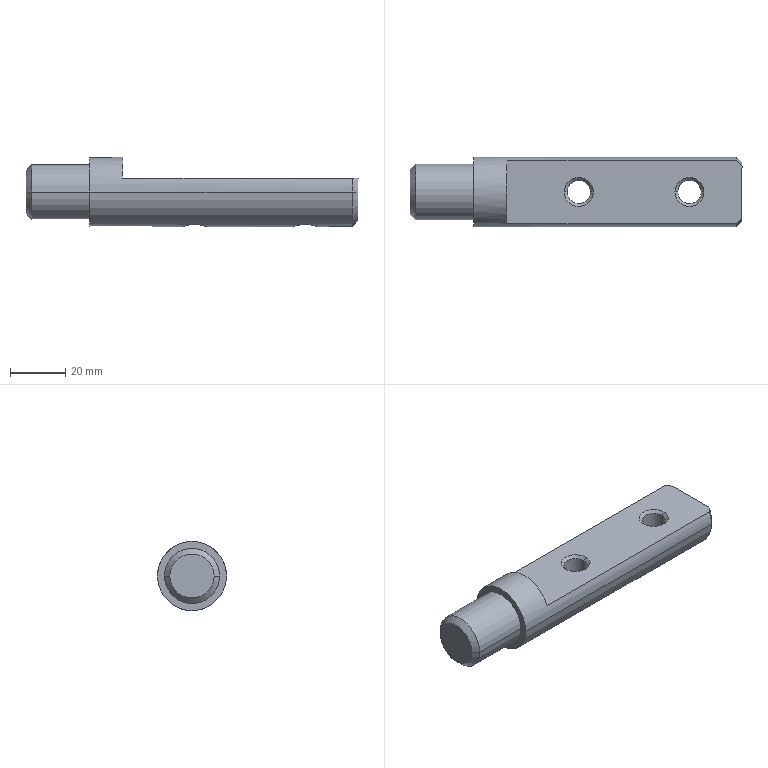Part | SolidWorks | features Chamfer 2, HoleWzd 1, ICE 1, Revolution 1 | 1 solid | 22 faces | box 120 x 25 x 25 mm | volume 42106 mm3 | cone 9 | cylinder 8 | plane 5 | commonest cylinder face diameters 8.5 x4 20 x2 25 x2
STEP:
#1=CARTESIAN_POINT('',(56.75,0.,4.));
#2=VERTEX_POINT('',#1);
#3=CARTESIAN_POINT('',(65.25,0.,4.));
#4=VERTEX_POINT('',#3);
#5=CARTESIAN_POINT('',(61.,0.,4.));
#6=DIRECTION('',(0.,0.,1.));
#7=DIRECTION('',(1.,0.,0.));
#8=AXIS2_PLACEMENT_3D('',#5,#6,#7);
#9=CIRCLE('',#8,4.25);
#10=EDGE_CURVE('',#2,#4,#9,.T.);
#11=ORIENTED_EDGE('',*,*,#10,.F.);
#12=CARTESIAN_POINT('',(55.75,0.,5.));
#13=VERTEX_POINT('',#12);
#14=CARTESIAN_POINT('',(56.75,0.,4.));
#15=DIRECTION('',(-0.7071,0.,0.7071));
#16=VECTOR('',#15,1000.);
#17=LINE('',#14,#16);
#18=EDGE_CURVE('',#2,#13,#17,.T.);
#19=ORIENTED_EDGE('',*,*,#18,.T.);
#20=CARTESIAN_POINT('',(66.25,0.,5.));
#21=VERTEX_POINT('',#20);
#22=CARTESIAN_POINT('',(61.,0.,5.));
#23=DIRECTION('',(0.,0.,-1.));
#24=DIRECTION('',(1.,0.,0.));
#25=AXIS2_PLACEMENT_3D('',#22,#23,#24);
#26=CIRCLE('',#25,5.25);
#27=EDGE_CURVE('',#21,#13,#26,.T.);
#28=ORIENTED_EDGE('',*,*,#27,.F.);
#29=CARTESIAN_POINT('',(65.25,0.,4.));
#30=DIRECTION('',(0.7071,0.,0.7071));
#31=VECTOR('',#30,1000.);
#32=LINE('',#29,#31);
#33=EDGE_CURVE('',#4,#21,#32,.T.);
#34=ORIENTED_EDGE('',*,*,#33,.F.);
#35=EDGE_LOOP('',(#11,#19,#28,#34));
#36=FACE_OUTER_BOUND('',#35,.T.);
#37=CARTESIAN_POINT('',(61.,0.,4.));
#38=DIRECTION('',(0.,0.,1.));
#39=DIRECTION('',(1.,0.,0.));
#40=AXIS2_PLACEMENT_3D('',#37,#38,#39);
#41=CONICAL_SURFACE('',#40,4.25,0.7854);
#42=ADVANCED_FACE('',(#36),#41,.F.);
#43=CARTESIAN_POINT('',(96.75,0.,4.));
#44=VERTEX_POINT('',#43);
#45=CARTESIAN_POINT('',(105.25,0.,4.));
#46=VERTEX_POINT('',#45);
#47=CARTESIAN_POINT('',(101.,0.,4.));
#48=DIRECTION('',(0.,0.,1.));
#49=DIRECTION('',(1.,0.,0.));
#50=AXIS2_PLACEMENT_3D('',#47,#48,#49);
#51=CIRCLE('',#50,4.25);
#52=EDGE_CURVE('',#44,#46,#51,.T.);
#53=ORIENTED_EDGE('',*,*,#52,.F.);
#54=CARTESIAN_POINT('',(95.75,0.,5.));
#55=VERTEX_POINT('',#54);
#56=CARTESIAN_POINT('',(96.75,0.,4.));
#57=DIRECTION('',(-0.7071,0.,0.7071));
#58=VECTOR('',#57,1000.);
#59=LINE('',#56,#58);
#60=EDGE_CURVE('',#44,#55,#59,.T.);
#61=ORIENTED_EDGE('',*,*,#60,.T.);
#62=CARTESIAN_POINT('',(106.25,0.,5.));
#63=VERTEX_POINT('',#62);
#64=CARTESIAN_POINT('',(101.,0.,5.));
#65=DIRECTION('',(0.,0.,-1.));
#66=DIRECTION('',(1.,0.,0.));
#67=AXIS2_PLACEMENT_3D('',#64,#65,#66);
#68=CIRCLE('',#67,5.25);
#69=EDGE_CURVE('',#63,#55,#68,.T.);
#70=ORIENTED_EDGE('',*,*,#69,.F.);
#71=CARTESIAN_POINT('',(105.25,0.,4.));
#72=DIRECTION('',(0.7071,0.,0.7071));
#73=VECTOR('',#72,1000.);
#74=LINE('',#71,#73);
#75=EDGE_CURVE('',#46,#63,#74,.T.);
#76=ORIENTED_EDGE('',*,*,#75,.F.);
#77=EDGE_LOOP('',(#53,#61,#70,#76));
#78=FACE_OUTER_BOUND('',#77,.T.);
#79=CARTESIAN_POINT('',(101.,0.,4.));
#80=DIRECTION('',(0.,0.,1.));
#81=DIRECTION('',(1.,0.,0.));
#82=AXIS2_PLACEMENT_3D('',#79,#80,#81);
#83=CONICAL_SURFACE('',#82,4.25,0.7854);
#84=ADVANCED_FACE('',(#78),#83,.F.);
#85=CARTESIAN_POINT('',(65.25,0.,-12.5));
#86=VERTEX_POINT('',#85);
#87=CARTESIAN_POINT('',(56.75,0.,-12.5));
#88=VERTEX_POINT('',#87);
#89=CARTESIAN_POINT('',(65.25,0.,-12.5));
#90=CARTESIAN_POINT('',(65.25,-0.2831,-12.5));
#91=CARTESIAN_POINT('',(65.222,-0.561,-12.49));
#92=CARTESIAN_POINT('',(65.113,-1.107,-12.454));
#93=CARTESIAN_POINT('',(65.03,-1.378,-12.426));
#94=CARTESIAN_POINT('',(64.816,-1.892,-12.359));
#95=CARTESIAN_POINT('',(64.685,-2.136,-12.318));
#96=CARTESIAN_POINT('',(64.376,-2.596,-12.23));
#97=CARTESIAN_POINT('',(64.198,-2.812,-12.181));
#98=CARTESIAN_POINT('',(63.809,-3.201,-12.085));
#99=CARTESIAN_POINT('',(63.597,-3.376,-12.037));
#100=CARTESIAN_POINT('',(63.133,-3.687,-11.945));
#101=CARTESIAN_POINT('',(62.889,-3.817,-11.903));
#102=CARTESIAN_POINT('',(62.379,-4.03,-11.833));
#103=CARTESIAN_POINT('',(62.109,-4.112,-11.804));
#104=CARTESIAN_POINT('',(61.559,-4.222,-11.765));
#105=CARTESIAN_POINT('',(61.282,-4.25,-11.755));
#106=CARTESIAN_POINT('',(60.723,-4.25,-11.755));
#107=CARTESIAN_POINT('',(60.439,-4.222,-11.766));
#108=CARTESIAN_POINT('',(59.892,-4.112,-11.804));
#109=CARTESIAN_POINT('',(59.626,-4.031,-11.833));
#110=CARTESIAN_POINT('',(59.108,-3.816,-11.904));
#111=CARTESIAN_POINT('',(58.864,-3.684,-11.946));
#112=CARTESIAN_POINT('',(58.405,-3.377,-12.036));
#113=CARTESIAN_POINT('',(58.189,-3.2,-12.085));
#114=CARTESIAN_POINT('',(57.798,-2.808,-12.182));
#115=CARTESIAN_POINT('',(57.624,-2.596,-12.23));
#116=CARTESIAN_POINT('',(57.316,-2.137,-12.318));
#117=CARTESIAN_POINT('',(57.182,-1.888,-12.359));
#118=CARTESIAN_POINT('',(56.97,-1.376,-12.427));
#119=CARTESIAN_POINT('',(56.888,-1.111,-12.454));
#120=CARTESIAN_POINT('',(56.778,-0.5605,-12.49));
#121=CARTESIAN_POINT('',(56.75,-0.2789,-12.5));
#122=CARTESIAN_POINT('',(56.75,0.,-12.5));
#123=B_SPLINE_CURVE_WITH_KNOTS('',3,(#89,#90,#91,#92,#93,#94,#95,#96,#97,#98,#99,#100,#101,#102,#103,#104,#105,#106,#107,#108,#109,#110,#111,#112,#113,#114,#115,#116,#117,#118,#119,#120,#121,#122),.UNSPECIFIED.,.F.,.F.,(4,2,2,2,2,2,2,2,2,2,2,2,2,2,2,2,4),(0.,0.0008368,0.001674,0.00251,0.003347,0.004184,0.005021,0.005857,0.006694,0.007531,0.008368,0.009204,0.01004,0.01088,0.01171,0.01255,0.01339),.UNSPECIFIED.);
#124=EDGE_CURVE('',#86,#88,#123,.T.);
#125=ORIENTED_EDGE('',*,*,#124,.T.);
#126=CARTESIAN_POINT('',(56.75,0.,5.));
#127=DIRECTION('',(0.,0.,1.));
#128=VECTOR('',#127,1000.);
#129=LINE('',#126,#128);
#130=EDGE_CURVE('',#88,#2,#129,.T.);
#131=ORIENTED_EDGE('',*,*,#130,.T.);
#132=ORIENTED_EDGE('',*,*,#10,.T.);
#133=CARTESIAN_POINT('',(65.25,0.,5.));
#134=DIRECTION('',(0.,0.,1.));
#135=VECTOR('',#134,1000.);
#136=LINE('',#133,#135);
#137=EDGE_CURVE('',#86,#4,#136,.T.);
#138=ORIENTED_EDGE('',*,*,#137,.F.);
#139=EDGE_LOOP('',(#125,#131,#132,#138));
#140=FACE_OUTER_BOUND('',#139,.T.);
#141=CARTESIAN_POINT('',(61.,0.,5.));
#142=DIRECTION('',(0.,0.,1.));
#143=DIRECTION('',(1.,0.,0.));
#144=AXIS2_PLACEMENT_3D('',#141,#142,#143);
#145=CYLINDRICAL_SURFACE('',#144,4.25);
#146=ADVANCED_FACE('',(#140),#145,.F.);
#147=CARTESIAN_POINT('',(105.25,0.,-12.5));
#148=VERTEX_POINT('',#147);
#149=CARTESIAN_POINT('',(96.75,0.,-12.5));
#150=VERTEX_POINT('',#149);
#151=CARTESIAN_POINT('',(105.25,0.,-12.5));
#152=CARTESIAN_POINT('',(105.25,-0.2831,-12.5));
#153=CARTESIAN_POINT('',(105.222,-0.561,-12.49));
#154=CARTESIAN_POINT('',(105.113,-1.107,-12.454));
#155=CARTESIAN_POINT('',(105.03,-1.378,-12.426));
#156=CARTESIAN_POINT('',(104.816,-1.892,-12.359));
#157=CARTESIAN_POINT('',(104.685,-2.136,-12.318));
#158=CARTESIAN_POINT('',(104.376,-2.596,-12.23));
#159=CARTESIAN_POINT('',(104.198,-2.812,-12.181));
#160=CARTESIAN_POINT('',(103.809,-3.201,-12.085));
#161=CARTESIAN_POINT('',(103.597,-3.376,-12.037));
#162=CARTESIAN_POINT('',(103.133,-3.687,-11.945));
#163=CARTESIAN_POINT('',(102.889,-3.817,-11.903));
#164=CARTESIAN_POINT('',(102.379,-4.03,-11.833));
#165=CARTESIAN_POINT('',(102.109,-4.112,-11.804));
#166=CARTESIAN_POINT('',(101.559,-4.222,-11.765));
#167=CARTESIAN_POINT('',(101.282,-4.25,-11.755));
#168=CARTESIAN_POINT('',(100.723,-4.25,-11.755));
#169=CARTESIAN_POINT('',(100.439,-4.222,-11.766));
#170=CARTESIAN_POINT('',(99.892,-4.112,-11.804));
#171=CARTESIAN_POINT('',(99.626,-4.031,-11.833));
#172=CARTESIAN_POINT('',(99.108,-3.816,-11.904));
#173=CARTESIAN_POINT('',(98.864,-3.684,-11.946));
#174=CARTESIAN_POINT('',(98.405,-3.377,-12.036));
#175=CARTESIAN_POINT('',(98.189,-3.2,-12.085));
#176=CARTESIAN_POINT('',(97.798,-2.808,-12.182));
#177=CARTESIAN_POINT('',(97.624,-2.596,-12.23));
#178=CARTESIAN_POINT('',(97.316,-2.137,-12.318));
#179=CARTESIAN_POINT('',(97.182,-1.888,-12.359));
#180=CARTESIAN_POINT('',(96.97,-1.376,-12.427));
#181=CARTESIAN_POINT('',(96.888,-1.111,-12.454));
#182=CARTESIAN_POINT('',(96.778,-0.5605,-12.49));
#183=CARTESIAN_POINT('',(96.75,-0.2789,-12.5));
#184=CARTESIAN_POINT('',(96.75,0.,-12.5));
#185=B_SPLINE_CURVE_WITH_KNOTS('',3,(#151,#152,#153,#154,#155,#156,#157,#158,#159,#160,#161,#162,#163,#164,#165,#166,#167,#168,#169,#170,#171,#172,#173,#174,#175,#176,#177,#178,#179,#180,#181,#182,#183,#184),.UNSPECIFIED.,.F.,.F.,(4,2,2,2,2,2,2,2,2,2,2,2,2,2,2,2,4),(0.,0.0008368,0.001674,0.00251,0.003347,0.004184,0.005021,0.005857,0.006694,0.007531,0.008368,0.009204,0.01004,0.01088,0.01171,0.01255,0.01339),.UNSPECIFIED.);
#186=EDGE_CURVE('',#148,#150,#185,.T.);
#187=ORIENTED_EDGE('',*,*,#186,.T.);
#188=CARTESIAN_POINT('',(96.75,0.,5.));
#189=DIRECTION('',(0.,0.,1.));
#190=VECTOR('',#189,1000.);
#191=LINE('',#188,#190);
#192=EDGE_CURVE('',#150,#44,#191,.T.);
#193=ORIENTED_EDGE('',*,*,#192,.T.);
#194=ORIENTED_EDGE('',*,*,#52,.T.);
#195=CARTESIAN_POINT('',(105.25,0.,5.));
#196=DIRECTION('',(0.,0.,1.));
#197=VECTOR('',#196,1000.);
#198=LINE('',#195,#197);
#199=EDGE_CURVE('',#148,#46,#198,.T.);
#200=ORIENTED_EDGE('',*,*,#199,.F.);
#201=EDGE_LOOP('',(#187,#193,#194,#200));
#202=FACE_OUTER_BOUND('',#201,.T.);
#203=CARTESIAN_POINT('',(101.,0.,5.));
#204=DIRECTION('',(0.,0.,1.));
#205=DIRECTION('',(1.,0.,0.));
#206=AXIS2_PLACEMENT_3D('',#203,#204,#205);
#207=CYLINDRICAL_SURFACE('',#206,4.25);
#208=ADVANCED_FACE('',(#202),#207,.F.);
#209=CARTESIAN_POINT('',(0.,-8.,0.));
#210=VERTEX_POINT('',#209);
#211=CARTESIAN_POINT('',(0.,8.,0.));
#212=VERTEX_POINT('',#211);
#213=CARTESIAN_POINT('',(0.,0.,0.));
#214=DIRECTION('',(-1.,0.,0.));
#215=DIRECTION('',(0.,-1.,0.));
#216=AXIS2_PLACEMENT_3D('',#213,#214,#215);
#217=CIRCLE('',#216,8.);
#218=EDGE_CURVE('',#210,#212,#217,.T.);
#219=ORIENTED_EDGE('',*,*,#218,.F.);
#220=CARTESIAN_POINT('',(2.,-10.,0.));
#221=VERTEX_POINT('',#220);
#222=CARTESIAN_POINT('',(2.,-10.,0.));
#223=DIRECTION('',(0.7071,-0.7071,0.));
#224=VECTOR('',#223,1000.);
#225=LINE('',#222,#224);
#226=EDGE_CURVE('',#210,#221,#225,.T.);
#227=ORIENTED_EDGE('',*,*,#226,.T.);
#228=CARTESIAN_POINT('',(2.,10.,0.));
#229=VERTEX_POINT('',#228);
#230=CARTESIAN_POINT('',(2.,0.,0.));
#231=DIRECTION('',(1.,0.,0.));
#232=DIRECTION('',(0.,-1.,0.));
#233=AXIS2_PLACEMENT_3D('',#230,#231,#232);
#234=CIRCLE('',#233,10.);
#235=EDGE_CURVE('',#229,#221,#234,.T.);
#236=ORIENTED_EDGE('',*,*,#235,.F.);
#237=CARTESIAN_POINT('',(2.,10.,0.));
#238=DIRECTION('',(0.7071,0.7071,0.));
#239=VECTOR('',#238,1000.);
#240=LINE('',#237,#239);
#241=EDGE_CURVE('',#212,#229,#240,.T.);
#242=ORIENTED_EDGE('',*,*,#241,.F.);
#243=EDGE_LOOP('',(#219,#227,#236,#242));
#244=FACE_OUTER_BOUND('',#243,.T.);
#245=CARTESIAN_POINT('',(2.,0.,0.));
#246=DIRECTION('',(1.,0.,0.));
#247=DIRECTION('',(0.,1.,0.));
#248=AXIS2_PLACEMENT_3D('',#245,#246,#247);
#249=CONICAL_SURFACE('',#248,10.,0.7854);
#250=ADVANCED_FACE('',(#244),#249,.T.);
#251=ORIENTED_EDGE('',*,*,#235,.T.);
#252=CARTESIAN_POINT('',(23.,-10.,0.));
#253=VERTEX_POINT('',#252);
#254=CARTESIAN_POINT('',(120.,-10.,0.));
#255=DIRECTION('',(1.,0.,0.));
#256=VECTOR('',#255,1000.);
#257=LINE('',#254,#256);
#258=EDGE_CURVE('',#221,#253,#257,.T.);
#259=ORIENTED_EDGE('',*,*,#258,.T.);
#260=CARTESIAN_POINT('',(23.,10.,0.));
#261=VERTEX_POINT('',#260);
#262=CARTESIAN_POINT('',(23.,0.,0.));
#263=DIRECTION('',(1.,0.,0.));
#264=DIRECTION('',(0.,1.,0.));
#265=AXIS2_PLACEMENT_3D('',#262,#263,#264);
#266=CIRCLE('',#265,10.);
#267=EDGE_CURVE('',#261,#253,#266,.T.);
#268=ORIENTED_EDGE('',*,*,#267,.F.);
#269=CARTESIAN_POINT('',(120.,10.,0.));
#270=DIRECTION('',(1.,0.,0.));
#271=VECTOR('',#270,1000.);
#272=LINE('',#269,#271);
#273=EDGE_CURVE('',#229,#261,#272,.T.);
#274=ORIENTED_EDGE('',*,*,#273,.F.);
#275=EDGE_LOOP('',(#251,#259,#268,#274));
#276=FACE_OUTER_BOUND('',#275,.T.);
#277=CARTESIAN_POINT('',(120.,0.,0.));
#278=DIRECTION('',(1.,0.,0.));
#279=DIRECTION('',(0.,1.,0.));
#280=AXIS2_PLACEMENT_3D('',#277,#278,#279);
#281=CYLINDRICAL_SURFACE('',#280,10.);
#282=ADVANCED_FACE('',(#276),#281,.T.);
#283=CARTESIAN_POINT('',(120.,10.5,0.));
#284=VERTEX_POINT('',#283);
#285=CARTESIAN_POINT('',(120.,9.233,5.));
#286=VERTEX_POINT('',#285);
#287=CARTESIAN_POINT('',(120.,0.,0.));
#288=DIRECTION('',(1.,0.,0.));
#289=DIRECTION('',(0.,1.,0.));
#290=AXIS2_PLACEMENT_3D('',#287,#288,#289);
#291=CIRCLE('',#290,10.5);
#292=EDGE_CURVE('',#284,#286,#291,.T.);
#293=ORIENTED_EDGE('',*,*,#292,.F.);
#294=CARTESIAN_POINT('',(118.,12.5,0.));
#295=VERTEX_POINT('',#294);
#296=CARTESIAN_POINT('',(120.,10.5,0.));
#297=DIRECTION('',(-0.7071,0.7071,0.));
#298=VECTOR('',#297,1000.);
#299=LINE('',#296,#298);
#300=EDGE_CURVE('',#284,#295,#299,.T.);
#301=ORIENTED_EDGE('',*,*,#300,.T.);
#302=CARTESIAN_POINT('',(118.,11.456,5.));
#303=VERTEX_POINT('',#302);
#304=CARTESIAN_POINT('',(118.,0.,0.));
#305=DIRECTION('',(-1.,0.,0.));
#306=DIRECTION('',(0.,1.,0.));
#307=AXIS2_PLACEMENT_3D('',#304,#305,#306);
#308=CIRCLE('',#307,12.5);
#309=EDGE_CURVE('',#303,#295,#308,.T.);
#310=ORIENTED_EDGE('',*,*,#309,.F.);
#311=CARTESIAN_POINT('',(118.,11.456,5.));
#312=CARTESIAN_POINT('',(118.674,10.722,5.));
#313=CARTESIAN_POINT('',(119.342,9.982,5.));
#314=CARTESIAN_POINT('',(120.,9.233,5.));
#315=B_SPLINE_CURVE_WITH_KNOTS('',3,(#311,#312,#313,#314),.UNSPECIFIED.,.F.,.F.,(4,4),(0.02169,0.02468),.UNSPECIFIED.);
#316=EDGE_CURVE('',#303,#286,#315,.T.);
#317=ORIENTED_EDGE('',*,*,#316,.T.);
#318=EDGE_LOOP('',(#293,#301,#310,#317));
#319=FACE_OUTER_BOUND('',#318,.T.);
#320=CARTESIAN_POINT('',(120.,0.,0.));
#321=DIRECTION('',(-1.,0.,0.));
#322=DIRECTION('',(0.,-1.,0.));
#323=AXIS2_PLACEMENT_3D('',#320,#321,#322);
#324=CONICAL_SURFACE('',#323,10.5,0.7854);
#325=ADVANCED_FACE('',(#319),#324,.T.);
#326=ORIENTED_EDGE('',*,*,#300,.F.);
#327=CARTESIAN_POINT('',(120.,-10.5,0.));
#328=VERTEX_POINT('',#327);
#329=CARTESIAN_POINT('',(120.,0.,0.));
#330=DIRECTION('',(1.,0.,0.));
#331=DIRECTION('',(0.,1.,0.));
#332=AXIS2_PLACEMENT_3D('',#329,#330,#331);
#333=CIRCLE('',#332,10.5);
#334=EDGE_CURVE('',#328,#284,#333,.T.);
#335=ORIENTED_EDGE('',*,*,#334,.F.);
#336=CARTESIAN_POINT('',(118.,-12.5,0.));
#337=VERTEX_POINT('',#336);
#338=CARTESIAN_POINT('',(120.,-10.5,0.));
#339=DIRECTION('',(-0.7071,-0.7071,0.));
#340=VECTOR('',#339,1000.);
#341=LINE('',#338,#340);
#342=EDGE_CURVE('',#328,#337,#341,.T.);
#343=ORIENTED_EDGE('',*,*,#342,.T.);
#344=CARTESIAN_POINT('',(118.,0.,0.));
#345=DIRECTION('',(-1.,0.,0.));
#346=DIRECTION('',(0.,1.,0.));
#347=AXIS2_PLACEMENT_3D('',#344,#345,#346);
#348=CIRCLE('',#347,12.5);
#349=EDGE_CURVE('',#295,#337,#348,.T.);
#350=ORIENTED_EDGE('',*,*,#349,.F.);
#351=EDGE_LOOP('',(#326,#335,#343,#350));
#352=FACE_OUTER_BOUND('',#351,.T.);
#353=CARTESIAN_POINT('',(120.,0.,0.));
#354=DIRECTION('',(-1.,0.,0.));
#355=DIRECTION('',(0.,-1.,0.));
#356=AXIS2_PLACEMENT_3D('',#353,#354,#355);
#357=CONICAL_SURFACE('',#356,10.5,0.7854);
#358=ADVANCED_FACE('',(#352),#357,.T.);
#359=CARTESIAN_POINT('',(23.,12.5,0.));
#360=VERTEX_POINT('',#359);
#361=CARTESIAN_POINT('',(23.,-12.5,0.));
#362=VERTEX_POINT('',#361);
#363=CARTESIAN_POINT('',(23.,0.,0.));
#364=DIRECTION('',(1.,0.,0.));
#365=DIRECTION('',(0.,1.,0.));
#366=AXIS2_PLACEMENT_3D('',#363,#364,#365);
#367=CIRCLE('',#366,12.5);
#368=EDGE_CURVE('',#360,#362,#367,.T.);
#369=ORIENTED_EDGE('',*,*,#368,.T.);
#370=CARTESIAN_POINT('',(120.,-12.5,0.));
#371=DIRECTION('',(1.,0.,0.));
#372=VECTOR('',#371,1000.);
#373=LINE('',#370,#372);
#374=EDGE_CURVE('',#362,#337,#373,.T.);
#375=ORIENTED_EDGE('',*,*,#374,.T.);
#376=CARTESIAN_POINT('',(118.,-11.456,5.));
#377=VERTEX_POINT('',#376);
#378=CARTESIAN_POINT('',(118.,0.,0.));
#379=DIRECTION('',(-1.,0.,0.));
#380=DIRECTION('',(0.,1.,0.));
#381=AXIS2_PLACEMENT_3D('',#378,#379,#380);
#382=CIRCLE('',#381,12.5);
#383=EDGE_CURVE('',#337,#377,#382,.T.);
#384=ORIENTED_EDGE('',*,*,#383,.T.);
#385=CARTESIAN_POINT('',(35.,-11.456,5.));
#386=VERTEX_POINT('',#385);
#387=CARTESIAN_POINT('',(120.,-11.456,5.));
#388=DIRECTION('',(-1.,0.,0.));
#389=VECTOR('',#388,1000.);
#390=LINE('',#387,#389);
#391=EDGE_CURVE('',#377,#386,#390,.T.);
#392=ORIENTED_EDGE('',*,*,#391,.T.);
#393=CARTESIAN_POINT('',(35.,11.456,5.));
#394=VERTEX_POINT('',#393);
#395=CARTESIAN_POINT('',(35.,0.,0.));
#396=DIRECTION('',(-1.,0.,0.));
#397=DIRECTION('',(0.,0.,-1.));
#398=AXIS2_PLACEMENT_3D('',#395,#396,#397);
#399=CIRCLE('',#398,12.5);
#400=EDGE_CURVE('',#386,#394,#399,.T.);
#401=ORIENTED_EDGE('',*,*,#400,.T.);
#402=CARTESIAN_POINT('',(120.,11.456,5.));
#403=DIRECTION('',(1.,0.,0.));
#404=VECTOR('',#403,1000.);
#405=LINE('',#402,#404);
#406=EDGE_CURVE('',#394,#303,#405,.T.);
#407=ORIENTED_EDGE('',*,*,#406,.T.);
#408=ORIENTED_EDGE('',*,*,#309,.T.);
#409=CARTESIAN_POINT('',(120.,12.5,0.));
#410=DIRECTION('',(1.,0.,0.));
#411=VECTOR('',#410,1000.);
#412=LINE('',#409,#411);
#413=EDGE_CURVE('',#360,#295,#412,.T.);
#414=ORIENTED_EDGE('',*,*,#413,.F.);
#415=EDGE_LOOP('',(#369,#375,#384,#392,#401,#407,#408,#414));
#416=FACE_OUTER_BOUND('',#415,.T.);
#417=CARTESIAN_POINT('',(120.,0.,0.));
#418=DIRECTION('',(1.,0.,0.));
#419=DIRECTION('',(0.,1.,0.));
#420=AXIS2_PLACEMENT_3D('',#417,#418,#419);
#421=CYLINDRICAL_SURFACE('',#420,12.5);
#422=ADVANCED_FACE('',(#416),#421,.T.);
#423=ORIENTED_EDGE('',*,*,#374,.F.);
#424=CARTESIAN_POINT('',(23.,0.,0.));
#425=DIRECTION('',(1.,0.,0.));
#426=DIRECTION('',(0.,1.,0.));
#427=AXIS2_PLACEMENT_3D('',#424,#425,#426);
#428=CIRCLE('',#427,12.5);
#429=EDGE_CURVE('',#362,#360,#428,.T.);
#430=ORIENTED_EDGE('',*,*,#429,.T.);
#431=ORIENTED_EDGE('',*,*,#413,.T.);
#432=ORIENTED_EDGE('',*,*,#349,.T.);
#433=EDGE_LOOP('',(#423,#430,#431,#432));
#434=FACE_OUTER_BOUND('',#433,.T.);
#435=ORIENTED_EDGE('',*,*,#124,.F.);
#436=CARTESIAN_POINT('',(56.75,0.,-12.5));
#437=CARTESIAN_POINT('',(56.75,0.2788,-12.5));
#438=CARTESIAN_POINT('',(56.778,0.5597,-12.491));
#439=CARTESIAN_POINT('',(56.888,1.111,-12.454));
#440=CARTESIAN_POINT('',(56.97,1.377,-12.427));
#441=CARTESIAN_POINT('',(57.183,1.89,-12.359));
#442=CARTESIAN_POINT('',(57.317,2.138,-12.318));
#443=CARTESIAN_POINT('',(57.624,2.597,-12.229));
#444=CARTESIAN_POINT('',(57.799,2.81,-12.182));
#445=CARTESIAN_POINT('',(58.388,3.398,-12.036));
#446=CARTESIAN_POINT('',(58.852,3.709,-11.939));
#447=CARTESIAN_POINT('',(59.626,4.031,-11.833));
#448=CARTESIAN_POINT('',(59.891,4.112,-11.804));
#449=CARTESIAN_POINT('',(60.437,4.222,-11.766));
#450=CARTESIAN_POINT('',(60.721,4.25,-11.755));
#451=CARTESIAN_POINT('',(61.281,4.25,-11.755));
#452=CARTESIAN_POINT('',(61.558,4.222,-11.765));
#453=CARTESIAN_POINT('',(62.108,4.113,-11.804));
#454=CARTESIAN_POINT('',(62.378,4.03,-11.833));
#455=CARTESIAN_POINT('',(62.89,3.817,-11.904));
#456=CARTESIAN_POINT('',(63.136,3.685,-11.946));
#457=CARTESIAN_POINT('',(63.598,3.375,-12.037));
#458=CARTESIAN_POINT('',(63.81,3.2,-12.085));
#459=CARTESIAN_POINT('',(64.2,2.811,-12.182));
#460=CARTESIAN_POINT('',(64.378,2.594,-12.23));
#461=CARTESIAN_POINT('',(64.685,2.135,-12.319));
#462=CARTESIAN_POINT('',(64.816,1.892,-12.359));
#463=CARTESIAN_POINT('',(65.03,1.378,-12.427));
#464=CARTESIAN_POINT('',(65.113,1.107,-12.454));
#465=CARTESIAN_POINT('',(65.222,0.561,-12.49));
#466=CARTESIAN_POINT('',(65.25,0.283,-12.5));
#467=CARTESIAN_POINT('',(65.25,0.,-12.5));
#468=B_SPLINE_CURVE_WITH_KNOTS('',3,(#436,#437,#438,#439,#440,#441,#442,#443,#444,#445,#446,#447,#448,#449,#450,#451,#452,#453,#454,#455,#456,#457,#458,#459,#460,#461,#462,#463,#464,#465,#466,#467),.UNSPECIFIED.,.F.,.F.,(4,2,2,2,2,2,2,2,2,2,2,2,2,2,2,4),(0.01339,0.01422,0.01506,0.0159,0.01673,0.01841,0.01924,0.02008,0.02092,0.02175,0.02259,0.02343,0.02426,0.0251,0.02594,0.02677),.UNSPECIFIED.);
#469=EDGE_CURVE('',#88,#86,#468,.T.);
#470=ORIENTED_EDGE('',*,*,#469,.F.);
#471=EDGE_LOOP('',(#435,#470));
#472=FACE_BOUND('',#471,.T.);
#473=ORIENTED_EDGE('',*,*,#186,.F.);
#474=CARTESIAN_POINT('',(96.75,0.,-12.5));
#475=CARTESIAN_POINT('',(96.75,0.2788,-12.5));
#476=CARTESIAN_POINT('',(96.778,0.5597,-12.491));
#477=CARTESIAN_POINT('',(96.888,1.111,-12.454));
#478=CARTESIAN_POINT('',(96.97,1.377,-12.427));
#479=CARTESIAN_POINT('',(97.183,1.89,-12.359));
#480=CARTESIAN_POINT('',(97.317,2.138,-12.318));
#481=CARTESIAN_POINT('',(97.624,2.597,-12.229));
#482=CARTESIAN_POINT('',(97.799,2.81,-12.182));
#483=CARTESIAN_POINT('',(98.388,3.398,-12.036));
#484=CARTESIAN_POINT('',(98.852,3.709,-11.939));
#485=CARTESIAN_POINT('',(99.626,4.031,-11.833));
#486=CARTESIAN_POINT('',(99.891,4.112,-11.804));
#487=CARTESIAN_POINT('',(100.437,4.222,-11.766));
#488=CARTESIAN_POINT('',(100.721,4.25,-11.755));
#489=CARTESIAN_POINT('',(101.281,4.25,-11.755));
#490=CARTESIAN_POINT('',(101.558,4.222,-11.765));
#491=CARTESIAN_POINT('',(102.108,4.113,-11.804));
#492=CARTESIAN_POINT('',(102.378,4.03,-11.833));
#493=CARTESIAN_POINT('',(102.89,3.817,-11.904));
#494=CARTESIAN_POINT('',(103.136,3.685,-11.946));
#495=CARTESIAN_POINT('',(103.598,3.375,-12.037));
#496=CARTESIAN_POINT('',(103.81,3.2,-12.085));
#497=CARTESIAN_POINT('',(104.2,2.811,-12.182));
#498=CARTESIAN_POINT('',(104.378,2.594,-12.23));
#499=CARTESIAN_POINT('',(104.685,2.135,-12.319));
#500=CARTESIAN_POINT('',(104.816,1.892,-12.359));
#501=CARTESIAN_POINT('',(105.03,1.378,-12.427));
#502=CARTESIAN_POINT('',(105.113,1.107,-12.454));
#503=CARTESIAN_POINT('',(105.222,0.561,-12.49));
#504=CARTESIAN_POINT('',(105.25,0.283,-12.5));
#505=CARTESIAN_POINT('',(105.25,0.,-12.5));
#506=B_SPLINE_CURVE_WITH_KNOTS('',3,(#474,#475,#476,#477,#478,#479,#480,#481,#482,#483,#484,#485,#486,#487,#488,#489,#490,#491,#492,#493,#494,#495,#496,#497,#498,#499,#500,#501,#502,#503,#504,#505),.UNSPECIFIED.,.F.,.F.,(4,2,2,2,2,2,2,2,2,2,2,2,2,2,2,4),(0.01339,0.01422,0.01506,0.0159,0.01673,0.01841,0.01924,0.02008,0.02092,0.02175,0.02259,0.02343,0.02426,0.0251,0.02594,0.02677),.UNSPECIFIED.);
#507=EDGE_CURVE('',#150,#148,#506,.T.);
#508=ORIENTED_EDGE('',*,*,#507,.F.);
#509=EDGE_LOOP('',(#473,#508));
#510=FACE_BOUND('',#509,.T.);
#511=CARTESIAN_POINT('',(120.,0.,0.));
#512=DIRECTION('',(1.,0.,0.));
#513=DIRECTION('',(0.,1.,0.));
#514=AXIS2_PLACEMENT_3D('',#511,#512,#513);
#515=CYLINDRICAL_SURFACE('',#514,12.5);
#516=ADVANCED_FACE('',(#434,#472,#510),#515,.T.);
#517=CARTESIAN_POINT('',(120.,-9.233,5.));
#518=VERTEX_POINT('',#517);
#519=CARTESIAN_POINT('',(120.,0.,0.));
#520=DIRECTION('',(1.,0.,0.));
#521=DIRECTION('',(0.,1.,0.));
#522=AXIS2_PLACEMENT_3D('',#519,#520,#521);
#523=CIRCLE('',#522,10.5);
#524=EDGE_CURVE('',#518,#328,#523,.T.);
#525=ORIENTED_EDGE('',*,*,#524,.T.);
#526=ORIENTED_EDGE('',*,*,#334,.T.);
#527=ORIENTED_EDGE('',*,*,#292,.T.);
#528=CARTESIAN_POINT('',(120.,12.5,5.));
#529=DIRECTION('',(0.,-1.,0.));
#530=VECTOR('',#529,1000.);
#531=LINE('',#528,#530);
#532=EDGE_CURVE('',#286,#518,#531,.T.);
#533=ORIENTED_EDGE('',*,*,#532,.T.);
#534=EDGE_LOOP('',(#525,#526,#527,#533));
#535=FACE_OUTER_BOUND('',#534,.T.);
#536=CARTESIAN_POINT('',(120.,12.5,0.));
#537=DIRECTION('',(1.,0.,0.));
#538=DIRECTION('',(0.,1.,0.));
#539=AXIS2_PLACEMENT_3D('',#536,#537,#538);
#540=PLANE('',#539);
#541=ADVANCED_FACE('',(#535),#540,.T.);
#542=ORIENTED_EDGE('',*,*,#342,.F.);
#543=ORIENTED_EDGE('',*,*,#524,.F.);
#544=CARTESIAN_POINT('',(120.,-9.233,5.));
#545=CARTESIAN_POINT('',(119.342,-9.982,5.));
#546=CARTESIAN_POINT('',(118.673,-10.722,5.));
#547=CARTESIAN_POINT('',(118.,-11.456,5.));
#548=B_SPLINE_CURVE_WITH_KNOTS('',3,(#544,#545,#546,#547),.UNSPECIFIED.,.F.,.F.,(4,4),(0.04626,0.04921),.UNSPECIFIED.);
#549=EDGE_CURVE('',#518,#377,#548,.T.);
#550=ORIENTED_EDGE('',*,*,#549,.T.);
#551=ORIENTED_EDGE('',*,*,#383,.F.);
#552=EDGE_LOOP('',(#542,#543,#550,#551));
#553=FACE_OUTER_BOUND('',#552,.T.);
#554=CARTESIAN_POINT('',(120.,0.,0.));
#555=DIRECTION('',(-1.,0.,0.));
#556=DIRECTION('',(0.,-1.,0.));
#557=AXIS2_PLACEMENT_3D('',#554,#555,#556);
#558=CONICAL_SURFACE('',#557,10.5,0.7854);
#559=ADVANCED_FACE('',(#553),#558,.T.);
#560=CARTESIAN_POINT('',(0.,0.,0.));
#561=DIRECTION('',(-1.,0.,0.));
#562=DIRECTION('',(0.,-1.,0.));
#563=AXIS2_PLACEMENT_3D('',#560,#561,#562);
#564=CIRCLE('',#563,8.);
#565=EDGE_CURVE('',#212,#210,#564,.T.);
#566=ORIENTED_EDGE('',*,*,#565,.T.);
#567=ORIENTED_EDGE('',*,*,#218,.T.);
#568=EDGE_LOOP('',(#566,#567));
#569=FACE_OUTER_BOUND('',#568,.T.);
#570=CARTESIAN_POINT('',(0.,0.,0.));
#571=DIRECTION('',(-1.,0.,0.));
#572=DIRECTION('',(0.,-1.,0.));
#573=AXIS2_PLACEMENT_3D('',#570,#571,#572);
#574=PLANE('',#573);
#575=ADVANCED_FACE('',(#569),#574,.T.);
#576=ORIENTED_EDGE('',*,*,#258,.F.);
#577=CARTESIAN_POINT('',(2.,0.,0.));
#578=DIRECTION('',(1.,0.,0.));
#579=DIRECTION('',(0.,-1.,0.));
#580=AXIS2_PLACEMENT_3D('',#577,#578,#579);
#581=CIRCLE('',#580,10.);
#582=EDGE_CURVE('',#221,#229,#581,.T.);
#583=ORIENTED_EDGE('',*,*,#582,.T.);
#584=ORIENTED_EDGE('',*,*,#273,.T.);
#585=CARTESIAN_POINT('',(23.,0.,0.));
#586=DIRECTION('',(1.,0.,0.));
#587=DIRECTION('',(0.,1.,0.));
#588=AXIS2_PLACEMENT_3D('',#585,#586,#587);
#589=CIRCLE('',#588,10.);
#590=EDGE_CURVE('',#253,#261,#589,.T.);
#591=ORIENTED_EDGE('',*,*,#590,.F.);
#592=EDGE_LOOP('',(#576,#583,#584,#591));
#593=FACE_OUTER_BOUND('',#592,.T.);
#594=CARTESIAN_POINT('',(120.,0.,0.));
#595=DIRECTION('',(1.,0.,0.));
#596=DIRECTION('',(0.,1.,0.));
#597=AXIS2_PLACEMENT_3D('',#594,#595,#596);
#598=CYLINDRICAL_SURFACE('',#597,10.);
#599=ADVANCED_FACE('',(#593),#598,.T.);
#600=ORIENTED_EDGE('',*,*,#267,.T.);
#601=ORIENTED_EDGE('',*,*,#590,.T.);
#602=EDGE_LOOP('',(#600,#601));
#603=FACE_BOUND('',#602,.T.);
#604=ORIENTED_EDGE('',*,*,#368,.F.);
#605=ORIENTED_EDGE('',*,*,#429,.F.);
#606=EDGE_LOOP('',(#604,#605));
#607=FACE_OUTER_BOUND('',#606,.T.);
#608=CARTESIAN_POINT('',(23.,12.5,0.));
#609=DIRECTION('',(-1.,0.,0.));
#610=DIRECTION('',(0.,-1.,0.));
#611=AXIS2_PLACEMENT_3D('',#608,#609,#610);
#612=PLANE('',#611);
#613=ADVANCED_FACE('',(#603,#607),#612,.T.);
#614=ORIENTED_EDGE('',*,*,#226,.F.);
#615=ORIENTED_EDGE('',*,*,#565,.F.);
#616=ORIENTED_EDGE('',*,*,#241,.T.);
#617=ORIENTED_EDGE('',*,*,#582,.F.);
#618=EDGE_LOOP('',(#614,#615,#616,#617));
#619=FACE_OUTER_BOUND('',#618,.T.);
#620=CARTESIAN_POINT('',(2.,0.,0.));
#621=DIRECTION('',(1.,0.,0.));
#622=DIRECTION('',(0.,1.,0.));
#623=AXIS2_PLACEMENT_3D('',#620,#621,#622);
#624=CONICAL_SURFACE('',#623,10.,0.7854);
#625=ADVANCED_FACE('',(#619),#624,.T.);
#626=CARTESIAN_POINT('',(35.,31.,5.));
#627=DIRECTION('',(0.,-1.,0.));
#628=VECTOR('',#627,1000.);
#629=LINE('',#626,#628);
#630=EDGE_CURVE('',#394,#386,#629,.T.);
#631=ORIENTED_EDGE('',*,*,#630,.F.);
#632=ORIENTED_EDGE('',*,*,#400,.F.);
#633=EDGE_LOOP('',(#631,#632));
#634=FACE_OUTER_BOUND('',#633,.T.);
#635=CARTESIAN_POINT('',(35.,31.,5.));
#636=DIRECTION('',(1.,0.,0.));
#637=DIRECTION('',(0.,0.,-1.));
#638=AXIS2_PLACEMENT_3D('',#635,#636,#637);
#639=PLANE('',#638);
#640=ADVANCED_FACE('',(#634),#639,.T.);
#641=ORIENTED_EDGE('',*,*,#69,.T.);
#642=CARTESIAN_POINT('',(101.,0.,5.));
#643=DIRECTION('',(0.,0.,-1.));
#644=DIRECTION('',(1.,0.,0.));
#645=AXIS2_PLACEMENT_3D('',#642,#643,#644);
#646=CIRCLE('',#645,5.25);
#647=EDGE_CURVE('',#55,#63,#646,.T.);
#648=ORIENTED_EDGE('',*,*,#647,.T.);
#649=EDGE_LOOP('',(#641,#648));
#650=FACE_BOUND('',#649,.T.);
#651=ORIENTED_EDGE('',*,*,#27,.T.);
#652=CARTESIAN_POINT('',(61.,0.,5.));
#653=DIRECTION('',(0.,0.,-1.));
#654=DIRECTION('',(1.,0.,0.));
#655=AXIS2_PLACEMENT_3D('',#652,#653,#654);
#656=CIRCLE('',#655,5.25);
#657=EDGE_CURVE('',#13,#21,#656,.T.);
#658=ORIENTED_EDGE('',*,*,#657,.T.);
#659=EDGE_LOOP('',(#651,#658));
#660=FACE_BOUND('',#659,.T.);
#661=ORIENTED_EDGE('',*,*,#630,.T.);
#662=ORIENTED_EDGE('',*,*,#391,.F.);
#663=ORIENTED_EDGE('',*,*,#549,.F.);
#664=ORIENTED_EDGE('',*,*,#532,.F.);
#665=ORIENTED_EDGE('',*,*,#316,.F.);
#666=ORIENTED_EDGE('',*,*,#406,.F.);
#667=EDGE_LOOP('',(#661,#662,#663,#664,#665,#666));
#668=FACE_OUTER_BOUND('',#667,.T.);
#669=CARTESIAN_POINT('',(35.,31.,5.));
#670=DIRECTION('',(0.,0.,1.));
#671=DIRECTION('',(1.,0.,0.));
#672=AXIS2_PLACEMENT_3D('',#669,#670,#671);
#673=PLANE('',#672);
#674=ADVANCED_FACE('',(#650,#660,#668),#673,.T.);
#675=ORIENTED_EDGE('',*,*,#192,.F.);
#676=ORIENTED_EDGE('',*,*,#507,.T.);
#677=ORIENTED_EDGE('',*,*,#199,.T.);
#678=CARTESIAN_POINT('',(101.,0.,4.));
#679=DIRECTION('',(0.,0.,1.));
#680=DIRECTION('',(1.,0.,0.));
#681=AXIS2_PLACEMENT_3D('',#678,#679,#680);
#682=CIRCLE('',#681,4.25);
#683=EDGE_CURVE('',#46,#44,#682,.T.);
#684=ORIENTED_EDGE('',*,*,#683,.T.);
#685=EDGE_LOOP('',(#675,#676,#677,#684));
#686=FACE_OUTER_BOUND('',#685,.T.);
#687=CARTESIAN_POINT('',(101.,0.,5.));
#688=DIRECTION('',(0.,0.,1.));
#689=DIRECTION('',(1.,0.,0.));
#690=AXIS2_PLACEMENT_3D('',#687,#688,#689);
#691=CYLINDRICAL_SURFACE('',#690,4.25);
#692=ADVANCED_FACE('',(#686),#691,.F.);
#693=ORIENTED_EDGE('',*,*,#130,.F.);
#694=ORIENTED_EDGE('',*,*,#469,.T.);
#695=ORIENTED_EDGE('',*,*,#137,.T.);
#696=CARTESIAN_POINT('',(61.,0.,4.));
#697=DIRECTION('',(0.,0.,1.));
#698=DIRECTION('',(1.,0.,0.));
#699=AXIS2_PLACEMENT_3D('',#696,#697,#698);
#700=CIRCLE('',#699,4.25);
#701=EDGE_CURVE('',#4,#2,#700,.T.);
#702=ORIENTED_EDGE('',*,*,#701,.T.);
#703=EDGE_LOOP('',(#693,#694,#695,#702));
#704=FACE_OUTER_BOUND('',#703,.T.);
#705=CARTESIAN_POINT('',(61.,0.,5.));
#706=DIRECTION('',(0.,0.,1.));
#707=DIRECTION('',(1.,0.,0.));
#708=AXIS2_PLACEMENT_3D('',#705,#706,#707);
#709=CYLINDRICAL_SURFACE('',#708,4.25);
#710=ADVANCED_FACE('',(#704),#709,.F.);
#711=ORIENTED_EDGE('',*,*,#60,.F.);
#712=ORIENTED_EDGE('',*,*,#683,.F.);
#713=ORIENTED_EDGE('',*,*,#75,.T.);
#714=ORIENTED_EDGE('',*,*,#647,.F.);
#715=EDGE_LOOP('',(#711,#712,#713,#714));
#716=FACE_OUTER_BOUND('',#715,.T.);
#717=CARTESIAN_POINT('',(101.,0.,4.));
#718=DIRECTION('',(0.,0.,1.));
#719=DIRECTION('',(1.,0.,0.));
#720=AXIS2_PLACEMENT_3D('',#717,#718,#719);
#721=CONICAL_SURFACE('',#720,4.25,0.7854);
#722=ADVANCED_FACE('',(#716),#721,.F.);
#723=ORIENTED_EDGE('',*,*,#18,.F.);
#724=ORIENTED_EDGE('',*,*,#701,.F.);
#725=ORIENTED_EDGE('',*,*,#33,.T.);
#726=ORIENTED_EDGE('',*,*,#657,.F.);
#727=EDGE_LOOP('',(#723,#724,#725,#726));
#728=FACE_OUTER_BOUND('',#727,.T.);
#729=CARTESIAN_POINT('',(61.,0.,4.));
#730=DIRECTION('',(0.,0.,1.));
#731=DIRECTION('',(1.,0.,0.));
#732=AXIS2_PLACEMENT_3D('',#729,#730,#731);
#733=CONICAL_SURFACE('',#732,4.25,0.7854);
#734=ADVANCED_FACE('',(#728),#733,.F.);
#735=CLOSED_SHELL('',(#42,#84,#146,#208,#250,#282,#325,#358,#422,#516,#541,#559,#575,#599,#613,#625,#640,#674,#692,#710,#722,#734));
#736=MANIFOLD_SOLID_BREP('',#735);
#737=CARTESIAN_POINT('',(0.,0.,0.));
#738=DIRECTION('',(0.,0.,1.));
#739=DIRECTION('',(1.,0.,0.));
#740=AXIS2_PLACEMENT_3D('',#737,#738,#739);
#741=(LENGTH_UNIT()NAMED_UNIT(*)SI_UNIT(.MILLI.,.METRE.));
#742=UNCERTAINTY_MEASURE_WITH_UNIT(LENGTH_MEASURE(0.00001),#741,'','');
#743=(NAMED_UNIT(*)PLANE_ANGLE_UNIT()SI_UNIT($,.RADIAN.));
#744=(NAMED_UNIT(*)SI_UNIT($,.STERADIAN.)SOLID_ANGLE_UNIT());
#745=(GEOMETRIC_REPRESENTATION_CONTEXT(3)GLOBAL_UNCERTAINTY_ASSIGNED_CONTEXT((#742))GLOBAL_UNIT_ASSIGNED_CONTEXT((#741,#743,#744))REPRESENTATION_CONTEXT('',''));
#746=ADVANCED_BREP_SHAPE_REPRESENTATION('',(#736,#740),#745);